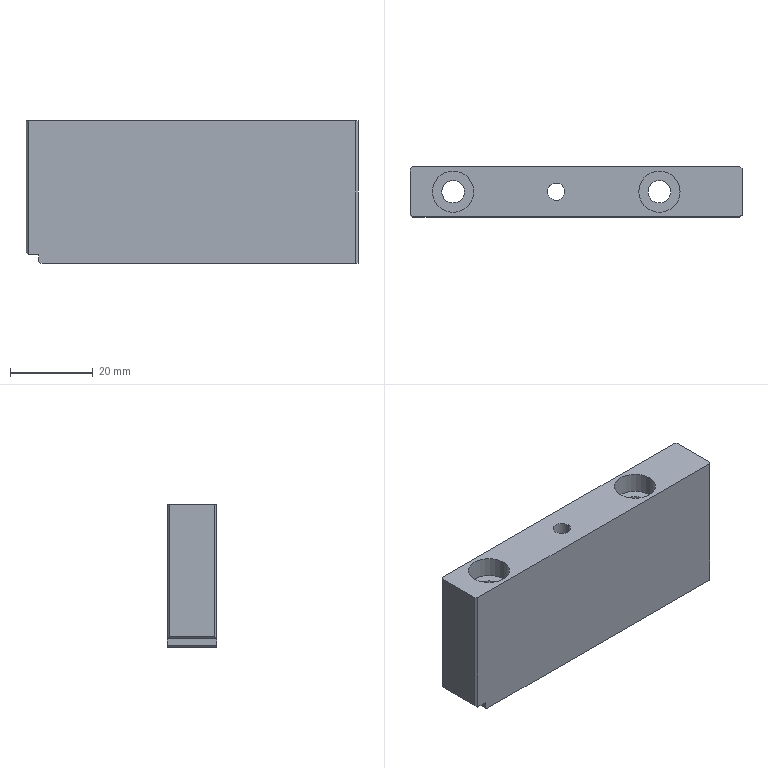Part | STEP file | side block 2 | 1 solid | 26 faces | box 80.434 x 12.1 x 34.5 mm | volume 30816 mm3 | plane 16 | cylinder 10 | commonest cylinder face diameters 5.5 x4 10 x4 4.2 x2